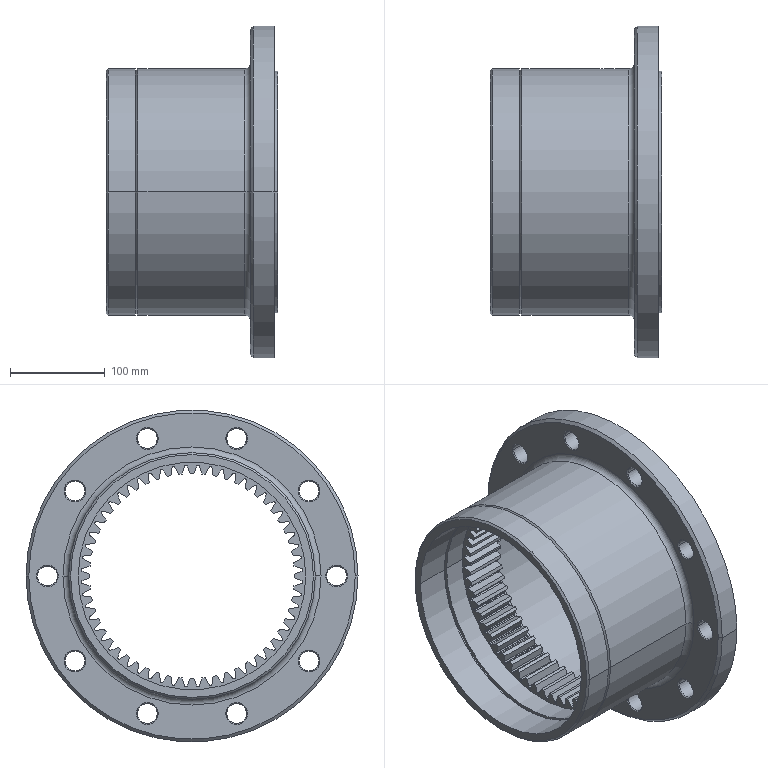Part | STEP file | Internal ring gear m=4  Z=56 | 1 solid | 492 faces | box 180.99 x 350 x 350 mm | volume 2653491 mm3 | cylinder 285 | spline 112 | plane 65 | cone 26 | torus 4 | commonest cylinder face diameters 3.04 x132 216 x57 234 x56 21 x20 240 x6 260 x4